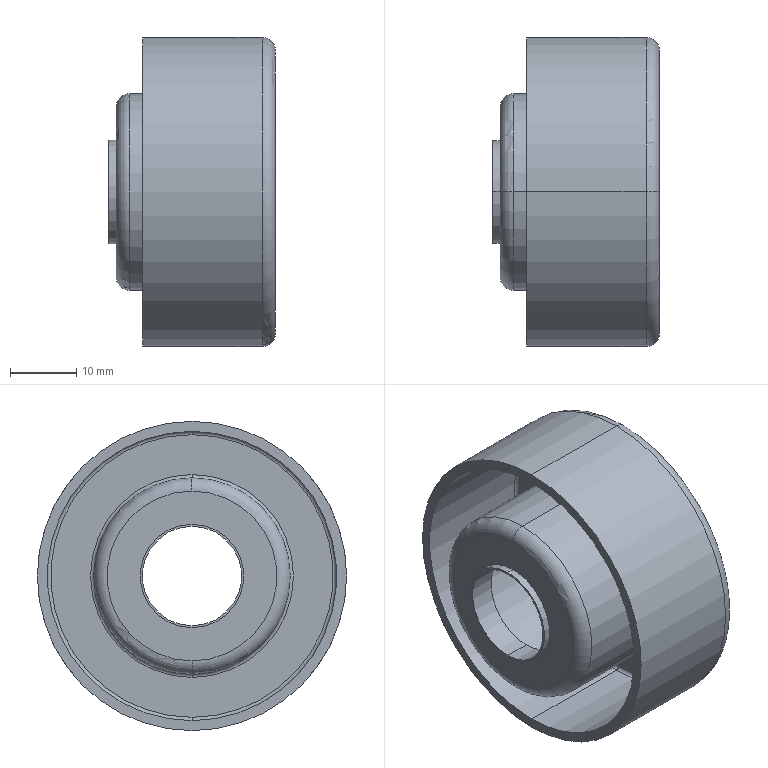Part | SolidWorks | features BaseBody 1 | 1 solid | 28 faces | box 25.129 x 46.6 x 46.6 mm | volume 9440 mm3 | cylinder 12 | torus 10 | plane 6 | commonest cylinder face diameters 15 x2 15.6 x2 26.6 x2 29.6 x2 43.6 x2 46.6 x2
STEP:
#1=CARTESIAN_POINT('',(-12.565,0.,2093.7));
#2=VERTEX_POINT('',#1);
#3=CARTESIAN_POINT('',(-12.565,0.,2109.3));
#4=VERTEX_POINT('',#3);
#5=CARTESIAN_POINT('',(-12.565,0.,2101.5));
#6=DIRECTION('',(1.,0.,0.));
#7=DIRECTION('',(0.,0.,-1.));
#8=AXIS2_PLACEMENT_3D('',#5,#6,#7);
#9=CIRCLE('',#8,7.8);
#10=EDGE_CURVE('',#2,#4,#9,.T.);
#11=ORIENTED_EDGE('',*,*,#10,.T.);
#12=CARTESIAN_POINT('',(-11.435,0.,2109.3));
#13=VERTEX_POINT('',#12);
#14=CARTESIAN_POINT('',(-25.285,0.,2109.3));
#15=DIRECTION('',(1.,0.,0.));
#16=VECTOR('',#15,1000.);
#17=LINE('',#14,#16);
#18=EDGE_CURVE('',#4,#13,#17,.T.);
#19=ORIENTED_EDGE('',*,*,#18,.T.);
#20=CARTESIAN_POINT('',(-11.435,0.,2093.7));
#21=VERTEX_POINT('',#20);
#22=CARTESIAN_POINT('',(-11.435,0.,2101.5));
#23=DIRECTION('',(1.,0.,0.));
#24=DIRECTION('',(0.,0.,-1.));
#25=AXIS2_PLACEMENT_3D('',#22,#23,#24);
#26=CIRCLE('',#25,7.8);
#27=EDGE_CURVE('',#21,#13,#26,.T.);
#28=ORIENTED_EDGE('',*,*,#27,.F.);
#29=CARTESIAN_POINT('',(-25.285,0.,2093.7));
#30=DIRECTION('',(1.,0.,0.));
#31=VECTOR('',#30,1000.);
#32=LINE('',#29,#31);
#33=EDGE_CURVE('',#2,#21,#32,.T.);
#34=ORIENTED_EDGE('',*,*,#33,.F.);
#35=EDGE_LOOP('',(#11,#19,#28,#34));
#36=FACE_OUTER_BOUND('',#35,.T.);
#37=CARTESIAN_POINT('',(-25.285,0.,2101.5));
#38=DIRECTION('',(1.,0.,0.));
#39=DIRECTION('',(0.,0.,-1.));
#40=AXIS2_PLACEMENT_3D('',#37,#38,#39);
#41=CYLINDRICAL_SURFACE('',#40,7.8);
#42=ADVANCED_FACE('',(#36),#41,.T.);
#43=CARTESIAN_POINT('',(-11.435,0.,2088.7));
#44=VERTEX_POINT('',#43);
#45=CARTESIAN_POINT('',(-11.435,0.,2114.3));
#46=VERTEX_POINT('',#45);
#47=CARTESIAN_POINT('',(-11.435,0.,2101.5));
#48=DIRECTION('',(1.,0.,0.));
#49=DIRECTION('',(0.,0.,-1.));
#50=AXIS2_PLACEMENT_3D('',#47,#48,#49);
#51=CIRCLE('',#50,12.8);
#52=EDGE_CURVE('',#44,#46,#51,.T.);
#53=ORIENTED_EDGE('',*,*,#52,.T.);
#54=CARTESIAN_POINT('',(-9.435,0.,2116.3));
#55=VERTEX_POINT('',#54);
#56=CARTESIAN_POINT('',(-9.435,0.,2114.3));
#57=DIRECTION('',(0.,1.,0.));
#58=DIRECTION('',(0.,0.,1.));
#59=AXIS2_PLACEMENT_3D('',#56,#57,#58);
#60=CIRCLE('',#59,2.);
#61=EDGE_CURVE('',#46,#55,#60,.T.);
#62=ORIENTED_EDGE('',*,*,#61,.T.);
#63=CARTESIAN_POINT('',(-9.435,0.,2086.7));
#64=VERTEX_POINT('',#63);
#65=CARTESIAN_POINT('',(-9.435,0.,2101.5));
#66=DIRECTION('',(1.,0.,0.));
#67=DIRECTION('',(0.,0.,-1.));
#68=AXIS2_PLACEMENT_3D('',#65,#66,#67);
#69=CIRCLE('',#68,14.8);
#70=EDGE_CURVE('',#64,#55,#69,.T.);
#71=ORIENTED_EDGE('',*,*,#70,.F.);
#72=CARTESIAN_POINT('',(-9.435,0.,2088.7));
#73=DIRECTION('',(0.,-1.,0.));
#74=DIRECTION('',(0.,0.,-1.));
#75=AXIS2_PLACEMENT_3D('',#72,#73,#74);
#76=CIRCLE('',#75,2.);
#77=EDGE_CURVE('',#44,#64,#76,.T.);
#78=ORIENTED_EDGE('',*,*,#77,.F.);
#79=EDGE_LOOP('',(#53,#62,#71,#78));
#80=FACE_OUTER_BOUND('',#79,.T.);
#81=CARTESIAN_POINT('',(-9.435,0.,2101.5));
#82=DIRECTION('',(1.,0.,0.));
#83=DIRECTION('',(0.,0.,-1.));
#84=AXIS2_PLACEMENT_3D('',#81,#82,#83);
#85=TOROIDAL_SURFACE('',#84,12.8,2.);
#86=ADVANCED_FACE('',(#80),#85,.T.);
#87=ORIENTED_EDGE('',*,*,#70,.T.);
#88=CARTESIAN_POINT('',(10.565,0.,2116.3));
#89=VERTEX_POINT('',#88);
#90=CARTESIAN_POINT('',(-25.285,0.,2116.3));
#91=DIRECTION('',(1.,0.,0.));
#92=VECTOR('',#91,1000.);
#93=LINE('',#90,#92);
#94=EDGE_CURVE('',#55,#89,#93,.T.);
#95=ORIENTED_EDGE('',*,*,#94,.T.);
#96=CARTESIAN_POINT('',(10.565,0.,2086.7));
#97=VERTEX_POINT('',#96);
#98=CARTESIAN_POINT('',(10.565,0.,2101.5));
#99=DIRECTION('',(1.,0.,0.));
#100=DIRECTION('',(0.,0.,-1.));
#101=AXIS2_PLACEMENT_3D('',#98,#99,#100);
#102=CIRCLE('',#101,14.8);
#103=EDGE_CURVE('',#97,#89,#102,.T.);
#104=ORIENTED_EDGE('',*,*,#103,.F.);
#105=CARTESIAN_POINT('',(-25.285,0.,2086.7));
#106=DIRECTION('',(1.,0.,0.));
#107=VECTOR('',#106,1000.);
#108=LINE('',#105,#107);
#109=EDGE_CURVE('',#64,#97,#108,.T.);
#110=ORIENTED_EDGE('',*,*,#109,.F.);
#111=EDGE_LOOP('',(#87,#95,#104,#110));
#112=FACE_OUTER_BOUND('',#111,.T.);
#113=CARTESIAN_POINT('',(-25.285,0.,2101.5));
#114=DIRECTION('',(1.,0.,0.));
#115=DIRECTION('',(0.,0.,-1.));
#116=AXIS2_PLACEMENT_3D('',#113,#114,#115);
#117=CYLINDRICAL_SURFACE('',#116,14.8);
#118=ADVANCED_FACE('',(#112),#117,.T.);
#119=CARTESIAN_POINT('',(11.065,0.,2116.8));
#120=VERTEX_POINT('',#119);
#121=CARTESIAN_POINT('',(11.065,0.,2086.2));
#122=VERTEX_POINT('',#121);
#123=CARTESIAN_POINT('',(11.065,0.,2101.5));
#124=DIRECTION('',(1.,0.,0.));
#125=DIRECTION('',(0.,0.,-1.));
#126=AXIS2_PLACEMENT_3D('',#123,#124,#125);
#127=CIRCLE('',#126,15.3);
#128=EDGE_CURVE('',#120,#122,#127,.T.);
#129=ORIENTED_EDGE('',*,*,#128,.F.);
#130=CARTESIAN_POINT('',(10.565,0.,2116.8));
#131=DIRECTION('',(0.,1.,0.));
#132=DIRECTION('',(0.,0.,1.));
#133=AXIS2_PLACEMENT_3D('',#130,#131,#132);
#134=CIRCLE('',#133,0.5);
#135=EDGE_CURVE('',#120,#89,#134,.T.);
#136=ORIENTED_EDGE('',*,*,#135,.T.);
#137=CARTESIAN_POINT('',(10.565,0.,2101.5));
#138=DIRECTION('',(1.,0.,0.));
#139=DIRECTION('',(0.,0.,-1.));
#140=AXIS2_PLACEMENT_3D('',#137,#138,#139);
#141=CIRCLE('',#140,14.8);
#142=EDGE_CURVE('',#89,#97,#141,.T.);
#143=ORIENTED_EDGE('',*,*,#142,.T.);
#144=CARTESIAN_POINT('',(10.565,0.,2086.2));
#145=DIRECTION('',(0.,-1.,0.));
#146=DIRECTION('',(0.,0.,-1.));
#147=AXIS2_PLACEMENT_3D('',#144,#145,#146);
#148=CIRCLE('',#147,0.5);
#149=EDGE_CURVE('',#122,#97,#148,.T.);
#150=ORIENTED_EDGE('',*,*,#149,.F.);
#151=EDGE_LOOP('',(#129,#136,#143,#150));
#152=FACE_OUTER_BOUND('',#151,.T.);
#153=CARTESIAN_POINT('',(10.565,0.,2101.5));
#154=DIRECTION('',(1.,0.,0.));
#155=DIRECTION('',(0.,0.,-1.));
#156=AXIS2_PLACEMENT_3D('',#153,#154,#155);
#157=TOROIDAL_SURFACE('',#156,15.3,0.5);
#158=ADVANCED_FACE('',(#152),#157,.F.);
#159=CARTESIAN_POINT('',(10.565,0.,2123.3));
#160=VERTEX_POINT('',#159);
#161=CARTESIAN_POINT('',(10.565,0.,2079.7));
#162=VERTEX_POINT('',#161);
#163=CARTESIAN_POINT('',(10.565,0.,2101.5));
#164=DIRECTION('',(1.,0.,0.));
#165=DIRECTION('',(0.,0.,-1.));
#166=AXIS2_PLACEMENT_3D('',#163,#164,#165);
#167=CIRCLE('',#166,21.8);
#168=EDGE_CURVE('',#160,#162,#167,.T.);
#169=ORIENTED_EDGE('',*,*,#168,.F.);
#170=CARTESIAN_POINT('',(11.065,0.,2122.8));
#171=VERTEX_POINT('',#170);
#172=CARTESIAN_POINT('',(10.565,0.,2122.8));
#173=DIRECTION('',(0.,1.,0.));
#174=DIRECTION('',(0.,0.,1.));
#175=AXIS2_PLACEMENT_3D('',#172,#173,#174);
#176=CIRCLE('',#175,0.5);
#177=EDGE_CURVE('',#160,#171,#176,.T.);
#178=ORIENTED_EDGE('',*,*,#177,.T.);
#179=CARTESIAN_POINT('',(11.065,0.,2080.2));
#180=VERTEX_POINT('',#179);
#181=CARTESIAN_POINT('',(11.065,0.,2101.5));
#182=DIRECTION('',(1.,0.,0.));
#183=DIRECTION('',(0.,0.,-1.));
#184=AXIS2_PLACEMENT_3D('',#181,#182,#183);
#185=CIRCLE('',#184,21.3);
#186=EDGE_CURVE('',#171,#180,#185,.T.);
#187=ORIENTED_EDGE('',*,*,#186,.T.);
#188=CARTESIAN_POINT('',(10.565,0.,2080.2));
#189=DIRECTION('',(0.,-1.,0.));
#190=DIRECTION('',(0.,0.,-1.));
#191=AXIS2_PLACEMENT_3D('',#188,#189,#190);
#192=CIRCLE('',#191,0.5);
#193=EDGE_CURVE('',#162,#180,#192,.T.);
#194=ORIENTED_EDGE('',*,*,#193,.F.);
#195=EDGE_LOOP('',(#169,#178,#187,#194));
#196=FACE_OUTER_BOUND('',#195,.T.);
#197=CARTESIAN_POINT('',(10.565,0.,2101.5));
#198=DIRECTION('',(1.,0.,0.));
#199=DIRECTION('',(0.,0.,-1.));
#200=AXIS2_PLACEMENT_3D('',#197,#198,#199);
#201=TOROIDAL_SURFACE('',#200,21.3,0.5);
#202=ADVANCED_FACE('',(#196),#201,.F.);
#203=CARTESIAN_POINT('',(-7.435,0.,2123.3));
#204=VERTEX_POINT('',#203);
#205=CARTESIAN_POINT('',(-7.435,0.,2079.7));
#206=VERTEX_POINT('',#205);
#207=CARTESIAN_POINT('',(-7.435,0.,2101.5));
#208=DIRECTION('',(1.,0.,0.));
#209=DIRECTION('',(0.,0.,-1.));
#210=AXIS2_PLACEMENT_3D('',#207,#208,#209);
#211=CIRCLE('',#210,21.8);
#212=EDGE_CURVE('',#204,#206,#211,.T.);
#213=ORIENTED_EDGE('',*,*,#212,.F.);
#214=CARTESIAN_POINT('',(-25.285,0.,2123.3));
#215=DIRECTION('',(1.,0.,0.));
#216=VECTOR('',#215,1000.);
#217=LINE('',#214,#216);
#218=EDGE_CURVE('',#204,#160,#217,.T.);
#219=ORIENTED_EDGE('',*,*,#218,.T.);
#220=ORIENTED_EDGE('',*,*,#168,.T.);
#221=CARTESIAN_POINT('',(-25.285,0.,2079.7));
#222=DIRECTION('',(1.,0.,0.));
#223=VECTOR('',#222,1000.);
#224=LINE('',#221,#223);
#225=EDGE_CURVE('',#206,#162,#224,.T.);
#226=ORIENTED_EDGE('',*,*,#225,.F.);
#227=EDGE_LOOP('',(#213,#219,#220,#226));
#228=FACE_OUTER_BOUND('',#227,.T.);
#229=CARTESIAN_POINT('',(-25.285,0.,2101.5));
#230=DIRECTION('',(1.,0.,0.));
#231=DIRECTION('',(0.,0.,-1.));
#232=AXIS2_PLACEMENT_3D('',#229,#230,#231);
#233=CYLINDRICAL_SURFACE('',#232,21.8);
#234=ADVANCED_FACE('',(#228),#233,.F.);
#235=CARTESIAN_POINT('',(-7.435,0.,2078.2));
#236=VERTEX_POINT('',#235);
#237=CARTESIAN_POINT('',(-7.435,0.,2124.8));
#238=VERTEX_POINT('',#237);
#239=CARTESIAN_POINT('',(-7.435,0.,2101.5));
#240=DIRECTION('',(1.,0.,0.));
#241=DIRECTION('',(0.,0.,-1.));
#242=AXIS2_PLACEMENT_3D('',#239,#240,#241);
#243=CIRCLE('',#242,23.3);
#244=EDGE_CURVE('',#236,#238,#243,.T.);
#245=ORIENTED_EDGE('',*,*,#244,.T.);
#246=CARTESIAN_POINT('',(10.565,0.,2124.8));
#247=VERTEX_POINT('',#246);
#248=CARTESIAN_POINT('',(-25.285,0.,2124.8));
#249=DIRECTION('',(1.,0.,0.));
#250=VECTOR('',#249,1000.);
#251=LINE('',#248,#250);
#252=EDGE_CURVE('',#238,#247,#251,.T.);
#253=ORIENTED_EDGE('',*,*,#252,.T.);
#254=CARTESIAN_POINT('',(10.565,0.,2078.2));
#255=VERTEX_POINT('',#254);
#256=CARTESIAN_POINT('',(10.565,0.,2101.5));
#257=DIRECTION('',(1.,0.,0.));
#258=DIRECTION('',(0.,0.,-1.));
#259=AXIS2_PLACEMENT_3D('',#256,#257,#258);
#260=CIRCLE('',#259,23.3);
#261=EDGE_CURVE('',#255,#247,#260,.T.);
#262=ORIENTED_EDGE('',*,*,#261,.F.);
#263=CARTESIAN_POINT('',(-25.285,0.,2078.2));
#264=DIRECTION('',(1.,0.,0.));
#265=VECTOR('',#264,1000.);
#266=LINE('',#263,#265);
#267=EDGE_CURVE('',#236,#255,#266,.T.);
#268=ORIENTED_EDGE('',*,*,#267,.F.);
#269=EDGE_LOOP('',(#245,#253,#262,#268));
#270=FACE_OUTER_BOUND('',#269,.T.);
#271=CARTESIAN_POINT('',(-25.285,0.,2101.5));
#272=DIRECTION('',(1.,0.,0.));
#273=DIRECTION('',(0.,0.,-1.));
#274=AXIS2_PLACEMENT_3D('',#271,#272,#273);
#275=CYLINDRICAL_SURFACE('',#274,23.3);
#276=ADVANCED_FACE('',(#270),#275,.T.);
#277=ORIENTED_EDGE('',*,*,#261,.T.);
#278=CARTESIAN_POINT('',(12.565,0.,2122.8));
#279=VERTEX_POINT('',#278);
#280=CARTESIAN_POINT('',(10.565,0.,2122.8));
#281=DIRECTION('',(0.,1.,0.));
#282=DIRECTION('',(0.,0.,1.));
#283=AXIS2_PLACEMENT_3D('',#280,#281,#282);
#284=CIRCLE('',#283,2.);
#285=EDGE_CURVE('',#247,#279,#284,.T.);
#286=ORIENTED_EDGE('',*,*,#285,.T.);
#287=CARTESIAN_POINT('',(12.565,0.,2080.2));
#288=VERTEX_POINT('',#287);
#289=CARTESIAN_POINT('',(12.565,0.,2101.5));
#290=DIRECTION('',(1.,0.,0.));
#291=DIRECTION('',(0.,0.,-1.));
#292=AXIS2_PLACEMENT_3D('',#289,#290,#291);
#293=CIRCLE('',#292,21.3);
#294=EDGE_CURVE('',#288,#279,#293,.T.);
#295=ORIENTED_EDGE('',*,*,#294,.F.);
#296=CARTESIAN_POINT('',(10.565,0.,2080.2));
#297=DIRECTION('',(0.,-1.,0.));
#298=DIRECTION('',(0.,0.,-1.));
#299=AXIS2_PLACEMENT_3D('',#296,#297,#298);
#300=CIRCLE('',#299,2.);
#301=EDGE_CURVE('',#255,#288,#300,.T.);
#302=ORIENTED_EDGE('',*,*,#301,.F.);
#303=EDGE_LOOP('',(#277,#286,#295,#302));
#304=FACE_OUTER_BOUND('',#303,.T.);
#305=CARTESIAN_POINT('',(10.565,0.,2101.5));
#306=DIRECTION('',(1.,0.,0.));
#307=DIRECTION('',(0.,0.,-1.));
#308=AXIS2_PLACEMENT_3D('',#305,#306,#307);
#309=TOROIDAL_SURFACE('',#308,21.3,2.);
#310=ADVANCED_FACE('',(#304),#309,.T.);
#311=CARTESIAN_POINT('',(12.565,0.,2086.2));
#312=VERTEX_POINT('',#311);
#313=CARTESIAN_POINT('',(12.565,0.,2116.8));
#314=VERTEX_POINT('',#313);
#315=CARTESIAN_POINT('',(12.565,0.,2101.5));
#316=DIRECTION('',(1.,0.,0.));
#317=DIRECTION('',(0.,0.,-1.));
#318=AXIS2_PLACEMENT_3D('',#315,#316,#317);
#319=CIRCLE('',#318,15.3);
#320=EDGE_CURVE('',#312,#314,#319,.T.);
#321=ORIENTED_EDGE('',*,*,#320,.T.);
#322=CARTESIAN_POINT('',(10.565,0.,2114.8));
#323=VERTEX_POINT('',#322);
#324=CARTESIAN_POINT('',(10.565,0.,2116.8));
#325=DIRECTION('',(0.,1.,0.));
#326=DIRECTION('',(0.,0.,1.));
#327=AXIS2_PLACEMENT_3D('',#324,#325,#326);
#328=CIRCLE('',#327,2.);
#329=EDGE_CURVE('',#314,#323,#328,.T.);
#330=ORIENTED_EDGE('',*,*,#329,.T.);
#331=CARTESIAN_POINT('',(10.565,0.,2088.2));
#332=VERTEX_POINT('',#331);
#333=CARTESIAN_POINT('',(10.565,0.,2101.5));
#334=DIRECTION('',(1.,0.,0.));
#335=DIRECTION('',(0.,0.,-1.));
#336=AXIS2_PLACEMENT_3D('',#333,#334,#335);
#337=CIRCLE('',#336,13.3);
#338=EDGE_CURVE('',#332,#323,#337,.T.);
#339=ORIENTED_EDGE('',*,*,#338,.F.);
#340=CARTESIAN_POINT('',(10.565,0.,2086.2));
#341=DIRECTION('',(0.,-1.,0.));
#342=DIRECTION('',(0.,0.,-1.));
#343=AXIS2_PLACEMENT_3D('',#340,#341,#342);
#344=CIRCLE('',#343,2.);
#345=EDGE_CURVE('',#312,#332,#344,.T.);
#346=ORIENTED_EDGE('',*,*,#345,.F.);
#347=EDGE_LOOP('',(#321,#330,#339,#346));
#348=FACE_OUTER_BOUND('',#347,.T.);
#349=CARTESIAN_POINT('',(10.565,0.,2101.5));
#350=DIRECTION('',(1.,0.,0.));
#351=DIRECTION('',(0.,0.,-1.));
#352=AXIS2_PLACEMENT_3D('',#349,#350,#351);
#353=TOROIDAL_SURFACE('',#352,15.3,2.);
#354=ADVANCED_FACE('',(#348),#353,.T.);
#355=CARTESIAN_POINT('',(-8.665,0.,2114.8));
#356=VERTEX_POINT('',#355);
#357=CARTESIAN_POINT('',(-8.665,0.,2088.2));
#358=VERTEX_POINT('',#357);
#359=CARTESIAN_POINT('',(-8.665,0.,2101.5));
#360=DIRECTION('',(1.,0.,0.));
#361=DIRECTION('',(0.,0.,-1.));
#362=AXIS2_PLACEMENT_3D('',#359,#360,#361);
#363=CIRCLE('',#362,13.3);
#364=EDGE_CURVE('',#356,#358,#363,.T.);
#365=ORIENTED_EDGE('',*,*,#364,.F.);
#366=CARTESIAN_POINT('',(-25.285,0.,2114.8));
#367=DIRECTION('',(1.,0.,0.));
#368=VECTOR('',#367,1000.);
#369=LINE('',#366,#368);
#370=EDGE_CURVE('',#356,#323,#369,.T.);
#371=ORIENTED_EDGE('',*,*,#370,.T.);
#372=CARTESIAN_POINT('',(10.565,0.,2101.5));
#373=DIRECTION('',(1.,0.,0.));
#374=DIRECTION('',(0.,0.,-1.));
#375=AXIS2_PLACEMENT_3D('',#372,#373,#374);
#376=CIRCLE('',#375,13.3);
#377=EDGE_CURVE('',#323,#332,#376,.T.);
#378=ORIENTED_EDGE('',*,*,#377,.T.);
#379=CARTESIAN_POINT('',(-25.285,0.,2088.2));
#380=DIRECTION('',(1.,0.,0.));
#381=VECTOR('',#380,1000.);
#382=LINE('',#379,#381);
#383=EDGE_CURVE('',#358,#332,#382,.T.);
#384=ORIENTED_EDGE('',*,*,#383,.F.);
#385=EDGE_LOOP('',(#365,#371,#378,#384));
#386=FACE_OUTER_BOUND('',#385,.T.);
#387=CARTESIAN_POINT('',(-25.285,0.,2101.5));
#388=DIRECTION('',(1.,0.,0.));
#389=DIRECTION('',(0.,0.,-1.));
#390=AXIS2_PLACEMENT_3D('',#387,#388,#389);
#391=CYLINDRICAL_SURFACE('',#390,13.3);
#392=ADVANCED_FACE('',(#386),#391,.F.);
#393=CARTESIAN_POINT('',(-12.565,0.,2109.));
#394=VERTEX_POINT('',#393);
#395=CARTESIAN_POINT('',(-12.565,0.,2094.));
#396=VERTEX_POINT('',#395);
#397=CARTESIAN_POINT('',(-12.565,0.,2101.5));
#398=DIRECTION('',(1.,0.,0.));
#399=DIRECTION('',(0.,0.,-1.));
#400=AXIS2_PLACEMENT_3D('',#397,#398,#399);
#401=CIRCLE('',#400,7.5);
#402=EDGE_CURVE('',#394,#396,#401,.T.);
#403=ORIENTED_EDGE('',*,*,#402,.F.);
#404=CARTESIAN_POINT('',(-8.665,0.,2109.));
#405=VERTEX_POINT('',#404);
#406=CARTESIAN_POINT('',(-25.285,0.,2109.));
#407=DIRECTION('',(1.,0.,0.));
#408=VECTOR('',#407,1000.);
#409=LINE('',#406,#408);
#410=EDGE_CURVE('',#394,#405,#409,.T.);
#411=ORIENTED_EDGE('',*,*,#410,.T.);
#412=CARTESIAN_POINT('',(-8.665,0.,2094.));
#413=VERTEX_POINT('',#412);
#414=CARTESIAN_POINT('',(-8.665,0.,2101.5));
#415=DIRECTION('',(1.,0.,0.));
#416=DIRECTION('',(0.,0.,-1.));
#417=AXIS2_PLACEMENT_3D('',#414,#415,#416);
#418=CIRCLE('',#417,7.5);
#419=EDGE_CURVE('',#405,#413,#418,.T.);
#420=ORIENTED_EDGE('',*,*,#419,.T.);
#421=CARTESIAN_POINT('',(-25.285,0.,2094.));
#422=DIRECTION('',(1.,0.,0.));
#423=VECTOR('',#422,1000.);
#424=LINE('',#421,#423);
#425=EDGE_CURVE('',#396,#413,#424,.T.);
#426=ORIENTED_EDGE('',*,*,#425,.F.);
#427=EDGE_LOOP('',(#403,#411,#420,#426));
#428=FACE_OUTER_BOUND('',#427,.T.);
#429=CARTESIAN_POINT('',(-25.285,0.,2101.5));
#430=DIRECTION('',(1.,0.,0.));
#431=DIRECTION('',(0.,0.,-1.));
#432=AXIS2_PLACEMENT_3D('',#429,#430,#431);
#433=CYLINDRICAL_SURFACE('',#432,7.5);
#434=ADVANCED_FACE('',(#428),#433,.F.);
#435=ORIENTED_EDGE('',*,*,#410,.F.);
#436=CARTESIAN_POINT('',(-12.565,0.,2101.5));
#437=DIRECTION('',(1.,0.,0.));
#438=DIRECTION('',(0.,0.,-1.));
#439=AXIS2_PLACEMENT_3D('',#436,#437,#438);
#440=CIRCLE('',#439,7.5);
#441=EDGE_CURVE('',#396,#394,#440,.T.);
#442=ORIENTED_EDGE('',*,*,#441,.F.);
#443=ORIENTED_EDGE('',*,*,#425,.T.);
#444=CARTESIAN_POINT('',(-8.665,0.,2101.5));
#445=DIRECTION('',(1.,0.,0.));
#446=DIRECTION('',(0.,0.,-1.));
#447=AXIS2_PLACEMENT_3D('',#444,#445,#446);
#448=CIRCLE('',#447,7.5);
#449=EDGE_CURVE('',#413,#405,#448,.T.);
#450=ORIENTED_EDGE('',*,*,#449,.T.);
#451=EDGE_LOOP('',(#435,#442,#443,#450));
#452=FACE_OUTER_BOUND('',#451,.T.);
#453=CARTESIAN_POINT('',(-25.285,0.,2101.5));
#454=DIRECTION('',(1.,0.,0.));
#455=DIRECTION('',(0.,0.,-1.));
#456=AXIS2_PLACEMENT_3D('',#453,#454,#455);
#457=CYLINDRICAL_SURFACE('',#456,7.5);
#458=ADVANCED_FACE('',(#452),#457,.F.);
#459=CARTESIAN_POINT('',(-8.665,0.,2101.5));
#460=DIRECTION('',(1.,0.,0.));
#461=DIRECTION('',(0.,0.,-1.));
#462=AXIS2_PLACEMENT_3D('',#459,#460,#461);
#463=CIRCLE('',#462,13.3);
#464=EDGE_CURVE('',#358,#356,#463,.T.);
#465=ORIENTED_EDGE('',*,*,#464,.T.);
#466=ORIENTED_EDGE('',*,*,#364,.T.);
#467=EDGE_LOOP('',(#465,#466));
#468=FACE_OUTER_BOUND('',#467,.T.);
#469=ORIENTED_EDGE('',*,*,#449,.F.);
#470=ORIENTED_EDGE('',*,*,#419,.F.);
#471=EDGE_LOOP('',(#469,#470));
#472=FACE_BOUND('',#471,.T.);
#473=CARTESIAN_POINT('',(-8.665,7.5,2101.5));
#474=DIRECTION('',(1.,0.,0.));
#475=DIRECTION('',(0.,0.,-1.));
#476=AXIS2_PLACEMENT_3D('',#473,#474,#475);
#477=PLANE('',#476);
#478=ADVANCED_FACE('',(#468,#472),#477,.T.);
#479=ORIENTED_EDGE('',*,*,#370,.F.);
#480=ORIENTED_EDGE('',*,*,#464,.F.);
#481=ORIENTED_EDGE('',*,*,#383,.T.);
#482=ORIENTED_EDGE('',*,*,#338,.T.);
#483=EDGE_LOOP('',(#479,#480,#481,#482));
#484=FACE_OUTER_BOUND('',#483,.T.);
#485=CARTESIAN_POINT('',(-25.285,0.,2101.5));
#486=DIRECTION('',(1.,0.,0.));
#487=DIRECTION('',(0.,0.,-1.));
#488=AXIS2_PLACEMENT_3D('',#485,#486,#487);
#489=CYLINDRICAL_SURFACE('',#488,13.3);
#490=ADVANCED_FACE('',(#484),#489,.F.);
#491=ORIENTED_EDGE('',*,*,#329,.F.);
#492=CARTESIAN_POINT('',(12.565,0.,2101.5));
#493=DIRECTION('',(1.,0.,0.));
#494=DIRECTION('',(0.,0.,-1.));
#495=AXIS2_PLACEMENT_3D('',#492,#493,#494);
#496=CIRCLE('',#495,15.3);
#497=EDGE_CURVE('',#314,#312,#496,.T.);
#498=ORIENTED_EDGE('',*,*,#497,.T.);
#499=ORIENTED_EDGE('',*,*,#345,.T.);
#500=ORIENTED_EDGE('',*,*,#377,.F.);
#501=EDGE_LOOP('',(#491,#498,#499,#500));
#502=FACE_OUTER_BOUND('',#501,.T.);
#503=CARTESIAN_POINT('',(10.565,0.,2101.5));
#504=DIRECTION('',(1.,0.,0.));
#505=DIRECTION('',(0.,0.,-1.));
#506=AXIS2_PLACEMENT_3D('',#503,#504,#505);
#507=TOROIDAL_SURFACE('',#506,15.3,2.);
#508=ADVANCED_FACE('',(#502),#507,.T.);
#509=ORIENTED_EDGE('',*,*,#294,.T.);
#510=CARTESIAN_POINT('',(12.565,0.,2101.5));
#511=DIRECTION('',(1.,0.,0.));
#512=DIRECTION('',(0.,0.,-1.));
#513=AXIS2_PLACEMENT_3D('',#510,#511,#512);
#514=CIRCLE('',#513,21.3);
#515=EDGE_CURVE('',#279,#288,#514,.T.);
#516=ORIENTED_EDGE('',*,*,#515,.T.);
#517=EDGE_LOOP('',(#509,#516));
#518=FACE_OUTER_BOUND('',#517,.T.);
#519=ORIENTED_EDGE('',*,*,#320,.F.);
#520=ORIENTED_EDGE('',*,*,#497,.F.);
#521=EDGE_LOOP('',(#519,#520));
#522=FACE_BOUND('',#521,.T.);
#523=CARTESIAN_POINT('',(12.565,15.3,2101.5));
#524=DIRECTION('',(1.,0.,0.));
#525=DIRECTION('',(0.,0.,-1.));
#526=AXIS2_PLACEMENT_3D('',#523,#524,#525);
#527=PLANE('',#526);
#528=ADVANCED_FACE('',(#518,#522),#527,.T.);
#529=ORIENTED_EDGE('',*,*,#285,.F.);
#530=CARTESIAN_POINT('',(10.565,0.,2101.5));
#531=DIRECTION('',(1.,0.,0.));
#532=DIRECTION('',(0.,0.,-1.));
#533=AXIS2_PLACEMENT_3D('',#530,#531,#532);
#534=CIRCLE('',#533,23.3);
#535=EDGE_CURVE('',#247,#255,#534,.T.);
#536=ORIENTED_EDGE('',*,*,#535,.T.);
#537=ORIENTED_EDGE('',*,*,#301,.T.);
#538=ORIENTED_EDGE('',*,*,#515,.F.);
#539=EDGE_LOOP('',(#529,#536,#537,#538));
#540=FACE_OUTER_BOUND('',#539,.T.);
#541=CARTESIAN_POINT('',(10.565,0.,2101.5));
#542=DIRECTION('',(1.,0.,0.));
#543=DIRECTION('',(0.,0.,-1.));
#544=AXIS2_PLACEMENT_3D('',#541,#542,#543);
#545=TOROIDAL_SURFACE('',#544,21.3,2.);
#546=ADVANCED_FACE('',(#540),#545,.T.);
#547=ORIENTED_EDGE('',*,*,#252,.F.);
#548=CARTESIAN_POINT('',(-7.435,0.,2101.5));
#549=DIRECTION('',(1.,0.,0.));
#550=DIRECTION('',(0.,0.,-1.));
#551=AXIS2_PLACEMENT_3D('',#548,#549,#550);
#552=CIRCLE('',#551,23.3);
#553=EDGE_CURVE('',#238,#236,#552,.T.);
#554=ORIENTED_EDGE('',*,*,#553,.T.);
#555=ORIENTED_EDGE('',*,*,#267,.T.);
#556=ORIENTED_EDGE('',*,*,#535,.F.);
#557=EDGE_LOOP('',(#547,#554,#555,#556));
#558=FACE_OUTER_BOUND('',#557,.T.);
#559=CARTESIAN_POINT('',(-25.285,0.,2101.5));
#560=DIRECTION('',(1.,0.,0.));
#561=DIRECTION('',(0.,0.,-1.));
#562=AXIS2_PLACEMENT_3D('',#559,#560,#561);
#563=CYLINDRICAL_SURFACE('',#562,23.3);
#564=ADVANCED_FACE('',(#558),#563,.T.);
#565=CARTESIAN_POINT('',(-7.435,0.,2101.5));
#566=DIRECTION('',(1.,0.,0.));
#567=DIRECTION('',(0.,0.,-1.));
#568=AXIS2_PLACEMENT_3D('',#565,#566,#567);
#569=CIRCLE('',#568,21.8);
#570=EDGE_CURVE('',#206,#204,#569,.T.);
#571=ORIENTED_EDGE('',*,*,#570,.T.);
#572=ORIENTED_EDGE('',*,*,#212,.T.);
#573=EDGE_LOOP('',(#571,#572));
#574=FACE_BOUND('',#573,.T.);
#575=ORIENTED_EDGE('',*,*,#244,.F.);
#576=ORIENTED_EDGE('',*,*,#553,.F.);
#577=EDGE_LOOP('',(#575,#576));
#578=FACE_OUTER_BOUND('',#577,.T.);
#579=CARTESIAN_POINT('',(-7.435,21.8,2101.5));
#580=DIRECTION('',(-1.,0.,0.));
#581=DIRECTION('',(0.,0.,1.));
#582=AXIS2_PLACEMENT_3D('',#579,#580,#581);
#583=PLANE('',#582);
#584=ADVANCED_FACE('',(#574,#578),#583,.T.);
#585=ORIENTED_EDGE('',*,*,#218,.F.);
#586=ORIENTED_EDGE('',*,*,#570,.F.);
#587=ORIENTED_EDGE('',*,*,#225,.T.);
#588=CARTESIAN_POINT('',(10.565,0.,2101.5));
#589=DIRECTION('',(1.,0.,0.));
#590=DIRECTION('',(0.,0.,-1.));
#591=AXIS2_PLACEMENT_3D('',#588,#589,#590);
#592=CIRCLE('',#591,21.8);
#593=EDGE_CURVE('',#162,#160,#592,.T.);
#594=ORIENTED_EDGE('',*,*,#593,.T.);
#595=EDGE_LOOP('',(#585,#586,#587,#594));
#596=FACE_OUTER_BOUND('',#595,.T.);
#597=CARTESIAN_POINT('',(-25.285,0.,2101.5));
#598=DIRECTION('',(1.,0.,0.));
#599=DIRECTION('',(0.,0.,-1.));
#600=AXIS2_PLACEMENT_3D('',#597,#598,#599);
#601=CYLINDRICAL_SURFACE('',#600,21.8);
#602=ADVANCED_FACE('',(#596),#601,.F.);
#603=ORIENTED_EDGE('',*,*,#177,.F.);
#604=ORIENTED_EDGE('',*,*,#593,.F.);
#605=ORIENTED_EDGE('',*,*,#193,.T.);
#606=CARTESIAN_POINT('',(11.065,0.,2101.5));
#607=DIRECTION('',(1.,0.,0.));
#608=DIRECTION('',(0.,0.,-1.));
#609=AXIS2_PLACEMENT_3D('',#606,#607,#608);
#610=CIRCLE('',#609,21.3);
#611=EDGE_CURVE('',#180,#171,#610,.T.);
#612=ORIENTED_EDGE('',*,*,#611,.T.);
#613=EDGE_LOOP('',(#603,#604,#605,#612));
#614=FACE_OUTER_BOUND('',#613,.T.);
#615=CARTESIAN_POINT('',(10.565,0.,2101.5));
#616=DIRECTION('',(1.,0.,0.));
#617=DIRECTION('',(0.,0.,-1.));
#618=AXIS2_PLACEMENT_3D('',#615,#616,#617);
#619=TOROIDAL_SURFACE('',#618,21.3,0.5);
#620=ADVANCED_FACE('',(#614),#619,.F.);
#621=CARTESIAN_POINT('',(11.065,0.,2101.5));
#622=DIRECTION('',(1.,0.,0.));
#623=DIRECTION('',(0.,0.,-1.));
#624=AXIS2_PLACEMENT_3D('',#621,#622,#623);
#625=CIRCLE('',#624,15.3);
#626=EDGE_CURVE('',#122,#120,#625,.T.);
#627=ORIENTED_EDGE('',*,*,#626,.T.);
#628=ORIENTED_EDGE('',*,*,#128,.T.);
#629=EDGE_LOOP('',(#627,#628));
#630=FACE_BOUND('',#629,.T.);
#631=ORIENTED_EDGE('',*,*,#611,.F.);
#632=ORIENTED_EDGE('',*,*,#186,.F.);
#633=EDGE_LOOP('',(#631,#632));
#634=FACE_OUTER_BOUND('',#633,.T.);
#635=CARTESIAN_POINT('',(11.065,21.3,2101.5));
#636=DIRECTION('',(-1.,0.,0.));
#637=DIRECTION('',(0.,0.,1.));
#638=AXIS2_PLACEMENT_3D('',#635,#636,#637);
#639=PLANE('',#638);
#640=ADVANCED_FACE('',(#630,#634),#639,.T.);
#641=ORIENTED_EDGE('',*,*,#135,.F.);
#642=ORIENTED_EDGE('',*,*,#626,.F.);
#643=ORIENTED_EDGE('',*,*,#149,.T.);
#644=ORIENTED_EDGE('',*,*,#103,.T.);
#645=EDGE_LOOP('',(#641,#642,#643,#644));
#646=FACE_OUTER_BOUND('',#645,.T.);
#647=CARTESIAN_POINT('',(10.565,0.,2101.5));
#648=DIRECTION('',(1.,0.,0.));
#649=DIRECTION('',(0.,0.,-1.));
#650=AXIS2_PLACEMENT_3D('',#647,#648,#649);
#651=TOROIDAL_SURFACE('',#650,15.3,0.5);
#652=ADVANCED_FACE('',(#646),#651,.F.);
#653=ORIENTED_EDGE('',*,*,#94,.F.);
#654=CARTESIAN_POINT('',(-9.435,0.,2101.5));
#655=DIRECTION('',(1.,0.,0.));
#656=DIRECTION('',(0.,0.,-1.));
#657=AXIS2_PLACEMENT_3D('',#654,#655,#656);
#658=CIRCLE('',#657,14.8);
#659=EDGE_CURVE('',#55,#64,#658,.T.);
#660=ORIENTED_EDGE('',*,*,#659,.T.);
#661=ORIENTED_EDGE('',*,*,#109,.T.);
#662=ORIENTED_EDGE('',*,*,#142,.F.);
#663=EDGE_LOOP('',(#653,#660,#661,#662));
#664=FACE_OUTER_BOUND('',#663,.T.);
#665=CARTESIAN_POINT('',(-25.285,0.,2101.5));
#666=DIRECTION('',(1.,0.,0.));
#667=DIRECTION('',(0.,0.,-1.));
#668=AXIS2_PLACEMENT_3D('',#665,#666,#667);
#669=CYLINDRICAL_SURFACE('',#668,14.8);
#670=ADVANCED_FACE('',(#664),#669,.T.);
#671=ORIENTED_EDGE('',*,*,#61,.F.);
#672=CARTESIAN_POINT('',(-11.435,0.,2101.5));
#673=DIRECTION('',(1.,0.,0.));
#674=DIRECTION('',(0.,0.,-1.));
#675=AXIS2_PLACEMENT_3D('',#672,#673,#674);
#676=CIRCLE('',#675,12.8);
#677=EDGE_CURVE('',#46,#44,#676,.T.);
#678=ORIENTED_EDGE('',*,*,#677,.T.);
#679=ORIENTED_EDGE('',*,*,#77,.T.);
#680=ORIENTED_EDGE('',*,*,#659,.F.);
#681=EDGE_LOOP('',(#671,#678,#679,#680));
#682=FACE_OUTER_BOUND('',#681,.T.);
#683=CARTESIAN_POINT('',(-9.435,0.,2101.5));
#684=DIRECTION('',(1.,0.,0.));
#685=DIRECTION('',(0.,0.,-1.));
#686=AXIS2_PLACEMENT_3D('',#683,#684,#685);
#687=TOROIDAL_SURFACE('',#686,12.8,2.);
#688=ADVANCED_FACE('',(#682),#687,.T.);
#689=ORIENTED_EDGE('',*,*,#27,.T.);
#690=CARTESIAN_POINT('',(-11.435,0.,2101.5));
#691=DIRECTION('',(1.,0.,0.));
#692=DIRECTION('',(0.,0.,-1.));
#693=AXIS2_PLACEMENT_3D('',#690,#691,#692);
#694=CIRCLE('',#693,7.8);
#695=EDGE_CURVE('',#13,#21,#694,.T.);
#696=ORIENTED_EDGE('',*,*,#695,.T.);
#697=EDGE_LOOP('',(#689,#696));
#698=FACE_BOUND('',#697,.T.);
#699=ORIENTED_EDGE('',*,*,#52,.F.);
#700=ORIENTED_EDGE('',*,*,#677,.F.);
#701=EDGE_LOOP('',(#699,#700));
#702=FACE_OUTER_BOUND('',#701,.T.);
#703=CARTESIAN_POINT('',(-11.435,12.8,2101.5));
#704=DIRECTION('',(-1.,0.,0.));
#705=DIRECTION('',(0.,0.,1.));
#706=AXIS2_PLACEMENT_3D('',#703,#704,#705);
#707=PLANE('',#706);
#708=ADVANCED_FACE('',(#698,#702),#707,.T.);
#709=ORIENTED_EDGE('',*,*,#18,.F.);
#710=CARTESIAN_POINT('',(-12.565,0.,2101.5));
#711=DIRECTION('',(1.,0.,0.));
#712=DIRECTION('',(0.,0.,-1.));
#713=AXIS2_PLACEMENT_3D('',#710,#711,#712);
#714=CIRCLE('',#713,7.8);
#715=EDGE_CURVE('',#4,#2,#714,.T.);
#716=ORIENTED_EDGE('',*,*,#715,.T.);
#717=ORIENTED_EDGE('',*,*,#33,.T.);
#718=ORIENTED_EDGE('',*,*,#695,.F.);
#719=EDGE_LOOP('',(#709,#716,#717,#718));
#720=FACE_OUTER_BOUND('',#719,.T.);
#721=CARTESIAN_POINT('',(-25.285,0.,2101.5));
#722=DIRECTION('',(1.,0.,0.));
#723=DIRECTION('',(0.,0.,-1.));
#724=AXIS2_PLACEMENT_3D('',#721,#722,#723);
#725=CYLINDRICAL_SURFACE('',#724,7.8);
#726=ADVANCED_FACE('',(#720),#725,.T.);
#727=ORIENTED_EDGE('',*,*,#441,.T.);
#728=ORIENTED_EDGE('',*,*,#402,.T.);
#729=EDGE_LOOP('',(#727,#728));
#730=FACE_BOUND('',#729,.T.);
#731=ORIENTED_EDGE('',*,*,#10,.F.);
#732=ORIENTED_EDGE('',*,*,#715,.F.);
#733=EDGE_LOOP('',(#731,#732));
#734=FACE_OUTER_BOUND('',#733,.T.);
#735=CARTESIAN_POINT('',(-12.565,7.8,2101.5));
#736=DIRECTION('',(-1.,0.,0.));
#737=DIRECTION('',(0.,0.,1.));
#738=AXIS2_PLACEMENT_3D('',#735,#736,#737);
#739=PLANE('',#738);
#740=ADVANCED_FACE('',(#730,#734),#739,.T.);
#741=CLOSED_SHELL('',(#42,#86,#118,#158,#202,#234,#276,#310,#354,#392,#434,#458,#478,#490,#508,#528,#546,#564,#584,#602,#620,#640,#652,#670,#688,#708,#726,#740));
#742=MANIFOLD_SOLID_BREP('',#741);
#743=CARTESIAN_POINT('',(0.,0.,0.));
#744=DIRECTION('',(0.,0.,1.));
#745=DIRECTION('',(1.,0.,0.));
#746=AXIS2_PLACEMENT_3D('',#743,#744,#745);
#747=(LENGTH_UNIT()NAMED_UNIT(*)SI_UNIT(.MILLI.,.METRE.));
#748=UNCERTAINTY_MEASURE_WITH_UNIT(LENGTH_MEASURE(0.00001),#747,'','');
#749=(NAMED_UNIT(*)PLANE_ANGLE_UNIT()SI_UNIT($,.RADIAN.));
#750=(NAMED_UNIT(*)SI_UNIT($,.STERADIAN.)SOLID_ANGLE_UNIT());
#751=(GEOMETRIC_REPRESENTATION_CONTEXT(3)GLOBAL_UNCERTAINTY_ASSIGNED_CONTEXT((#748))GLOBAL_UNIT_ASSIGNED_CONTEXT((#747,#749,#750))REPRESENTATION_CONTEXT('',''));
#752=ADVANCED_BREP_SHAPE_REPRESENTATION('',(#742,#746),#751);